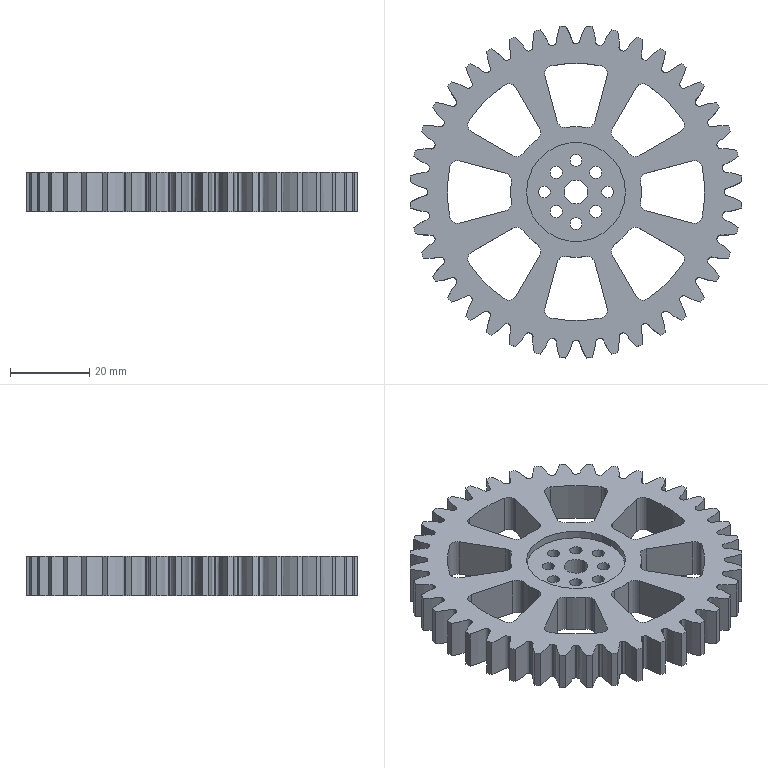Part | STEP file | FD gear 40 | 1 solid | 256 faces | box 83.847 x 83.847 x 10 mm | volume 32005 mm3 | cylinder 157 | spline 80 | plane 19 | commonest cylinder face diameters 75 x41 4 x40 84 x40 3 x8 3.1 x8 33 x8